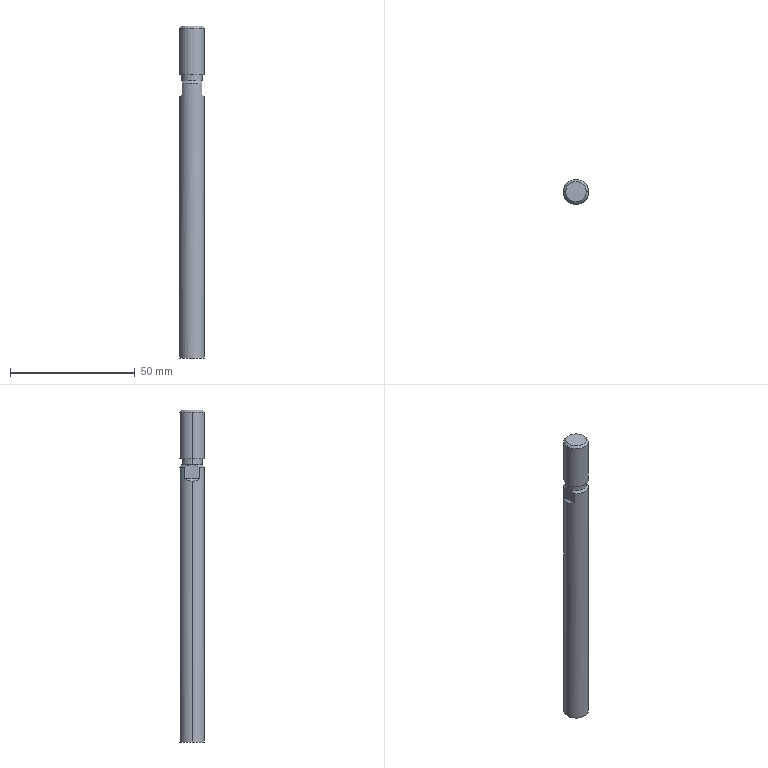Part | STEP file | rod_A_CDM2B25_100_C76_0_ | 1 solid | 19 faces | box 10 x 10 x 133 mm | volume 10311 mm3 | plane 9 | cylinder 6 | cone 4 | commonest cylinder face diameters 10 x4 8.16 x2
STEP:
#1=CARTESIAN_POINT('',(5.,0.,-101.));
#2=VERTEX_POINT('',#1);
#3=CARTESIAN_POINT('',(-5.,0.,-101.));
#4=VERTEX_POINT('',#3);
#5=CARTESIAN_POINT('',(0.,0.,-101.));
#6=DIRECTION('',(0.,0.,1.));
#7=DIRECTION('',(1.,0.,0.));
#8=AXIS2_PLACEMENT_3D('',#5,#6,#7);
#9=CIRCLE('',#8,5.);
#10=EDGE_CURVE('',#2,#4,#9,.T.);
#11=ORIENTED_EDGE('',*,*,#10,.T.);
#12=CARTESIAN_POINT('',(-5.,0.,3.5));
#13=VERTEX_POINT('',#12);
#14=CARTESIAN_POINT('',(-5.,0.,-101.));
#15=DIRECTION('',(0.,0.,1.));
#16=VECTOR('',#15,1000.);
#17=LINE('',#14,#16);
#18=EDGE_CURVE('',#4,#13,#17,.T.);
#19=ORIENTED_EDGE('',*,*,#18,.T.);
#20=CARTESIAN_POINT('',(-4.,3.,4.5));
#21=VERTEX_POINT('',#20);
#22=CARTESIAN_POINT('',(-5.,0.,3.5));
#23=CARTESIAN_POINT('',(-5.,1.091,3.5));
#24=CARTESIAN_POINT('',(-4.655,2.127,3.845));
#25=CARTESIAN_POINT('',(-4.,3.,4.5));
#26=(BOUNDED_CURVE()B_SPLINE_CURVE(3,(#22,#23,#24,#25),.UNSPECIFIED.,.F.,.T.)B_SPLINE_CURVE_WITH_KNOTS((4,4),(3.142,3.785),.UNSPECIFIED.)CURVE()GEOMETRIC_REPRESENTATION_ITEM()RATIONAL_B_SPLINE_CURVE((1.,0.9658,0.9658,1.))REPRESENTATION_ITEM(''));
#27=EDGE_CURVE('',#13,#21,#26,.T.);
#28=ORIENTED_EDGE('',*,*,#27,.T.);
#29=CARTESIAN_POINT('',(-4.,3.,9.08));
#30=VERTEX_POINT('',#29);
#31=CARTESIAN_POINT('',(-4.,3.,-101.));
#32=DIRECTION('',(0.,0.,1.));
#33=VECTOR('',#32,1000.);
#34=LINE('',#31,#33);
#35=EDGE_CURVE('',#21,#30,#34,.T.);
#36=ORIENTED_EDGE('',*,*,#35,.T.);
#37=CARTESIAN_POINT('',(4.,3.,9.08));
#38=VERTEX_POINT('',#37);
#39=CARTESIAN_POINT('',(0.,0.,9.08));
#40=DIRECTION('',(0.,0.,1.));
#41=DIRECTION('',(1.,0.,0.));
#42=AXIS2_PLACEMENT_3D('',#39,#40,#41);
#43=CIRCLE('',#42,5.);
#44=EDGE_CURVE('',#38,#30,#43,.T.);
#45=ORIENTED_EDGE('',*,*,#44,.F.);
#46=CARTESIAN_POINT('',(4.,3.,4.5));
#47=VERTEX_POINT('',#46);
#48=CARTESIAN_POINT('',(4.,3.,-101.));
#49=DIRECTION('',(0.,0.,-1.));
#50=VECTOR('',#49,1000.);
#51=LINE('',#48,#50);
#52=EDGE_CURVE('',#38,#47,#51,.T.);
#53=ORIENTED_EDGE('',*,*,#52,.T.);
#54=CARTESIAN_POINT('',(5.,0.,3.5));
#55=VERTEX_POINT('',#54);
#56=CARTESIAN_POINT('',(4.,3.,4.5));
#57=CARTESIAN_POINT('',(4.655,2.127,3.845));
#58=CARTESIAN_POINT('',(5.,1.091,3.5));
#59=CARTESIAN_POINT('',(5.,0.,3.5));
#60=(BOUNDED_CURVE()B_SPLINE_CURVE(3,(#56,#57,#58,#59),.UNSPECIFIED.,.F.,.T.)B_SPLINE_CURVE_WITH_KNOTS((4,4),(2.498,3.142),.UNSPECIFIED.)CURVE()GEOMETRIC_REPRESENTATION_ITEM()RATIONAL_B_SPLINE_CURVE((1.,0.9658,0.9658,1.))REPRESENTATION_ITEM(''));
#61=EDGE_CURVE('',#47,#55,#60,.T.);
#62=ORIENTED_EDGE('',*,*,#61,.T.);
#63=CARTESIAN_POINT('',(5.,0.,-101.));
#64=DIRECTION('',(0.,0.,1.));
#65=VECTOR('',#64,1000.);
#66=LINE('',#63,#65);
#67=EDGE_CURVE('',#2,#55,#66,.T.);
#68=ORIENTED_EDGE('',*,*,#67,.F.);
#69=EDGE_LOOP('',(#11,#19,#28,#36,#45,#53,#62,#68));
#70=FACE_OUTER_BOUND('',#69,.T.);
#71=CARTESIAN_POINT('',(0.,0.,-101.));
#72=DIRECTION('',(0.,0.,1.));
#73=DIRECTION('',(1.,0.,0.));
#74=AXIS2_PLACEMENT_3D('',#71,#72,#73);
#75=CYLINDRICAL_SURFACE('',#74,5.);
#76=ADVANCED_FACE('',(#70),#75,.T.);
#77=CARTESIAN_POINT('',(-4.,0.804,10.));
#78=VERTEX_POINT('',#77);
#79=CARTESIAN_POINT('',(-4.08,0.,10.));
#80=VERTEX_POINT('',#79);
#81=CARTESIAN_POINT('',(0.,0.,10.));
#82=DIRECTION('',(0.,0.,1.));
#83=DIRECTION('',(1.,0.,0.));
#84=AXIS2_PLACEMENT_3D('',#81,#82,#83);
#85=CIRCLE('',#84,4.08);
#86=EDGE_CURVE('',#78,#80,#85,.T.);
#87=ORIENTED_EDGE('',*,*,#86,.T.);
#88=CARTESIAN_POINT('',(-4.08,0.,12.5));
#89=VERTEX_POINT('',#88);
#90=CARTESIAN_POINT('',(-4.08,0.,-101.));
#91=DIRECTION('',(0.,0.,1.));
#92=VECTOR('',#91,1000.);
#93=LINE('',#90,#92);
#94=EDGE_CURVE('',#80,#89,#93,.T.);
#95=ORIENTED_EDGE('',*,*,#94,.T.);
#96=CARTESIAN_POINT('',(4.08,0.,12.5));
#97=VERTEX_POINT('',#96);
#98=CARTESIAN_POINT('',(0.,0.,12.5));
#99=DIRECTION('',(0.,0.,1.));
#100=DIRECTION('',(1.,0.,0.));
#101=AXIS2_PLACEMENT_3D('',#98,#99,#100);
#102=CIRCLE('',#101,4.08);
#103=EDGE_CURVE('',#97,#89,#102,.T.);
#104=ORIENTED_EDGE('',*,*,#103,.F.);
#105=CARTESIAN_POINT('',(4.08,0.,10.));
#106=VERTEX_POINT('',#105);
#107=CARTESIAN_POINT('',(4.08,0.,-101.));
#108=DIRECTION('',(0.,0.,1.));
#109=VECTOR('',#108,1000.);
#110=LINE('',#107,#109);
#111=EDGE_CURVE('',#106,#97,#110,.T.);
#112=ORIENTED_EDGE('',*,*,#111,.F.);
#113=CARTESIAN_POINT('',(4.,0.804,10.));
#114=VERTEX_POINT('',#113);
#115=CARTESIAN_POINT('',(0.,0.,10.));
#116=DIRECTION('',(0.,0.,1.));
#117=DIRECTION('',(1.,0.,0.));
#118=AXIS2_PLACEMENT_3D('',#115,#116,#117);
#119=CIRCLE('',#118,4.08);
#120=EDGE_CURVE('',#106,#114,#119,.T.);
#121=ORIENTED_EDGE('',*,*,#120,.T.);
#122=CARTESIAN_POINT('',(0.,0.,10.));
#123=DIRECTION('',(0.,0.,1.));
#124=DIRECTION('',(1.,0.,0.));
#125=AXIS2_PLACEMENT_3D('',#122,#123,#124);
#126=CIRCLE('',#125,4.08);
#127=EDGE_CURVE('',#114,#78,#126,.T.);
#128=ORIENTED_EDGE('',*,*,#127,.T.);
#129=EDGE_LOOP('',(#87,#95,#104,#112,#121,#128));
#130=FACE_OUTER_BOUND('',#129,.T.);
#131=CARTESIAN_POINT('',(0.,0.,-101.));
#132=DIRECTION('',(0.,0.,1.));
#133=DIRECTION('',(1.,0.,0.));
#134=AXIS2_PLACEMENT_3D('',#131,#132,#133);
#135=CYLINDRICAL_SURFACE('',#134,4.08);
#136=ADVANCED_FACE('',(#130),#135,.T.);
#137=CARTESIAN_POINT('',(5.,0.,12.5));
#138=VERTEX_POINT('',#137);
#139=CARTESIAN_POINT('',(-5.,0.,12.5));
#140=VERTEX_POINT('',#139);
#141=CARTESIAN_POINT('',(0.,0.,12.5));
#142=DIRECTION('',(0.,0.,1.));
#143=DIRECTION('',(1.,0.,0.));
#144=AXIS2_PLACEMENT_3D('',#141,#142,#143);
#145=CIRCLE('',#144,5.);
#146=EDGE_CURVE('',#138,#140,#145,.T.);
#147=ORIENTED_EDGE('',*,*,#146,.T.);
#148=CARTESIAN_POINT('',(-5.,0.,31.08));
#149=VERTEX_POINT('',#148);
#150=CARTESIAN_POINT('',(-5.,0.,-101.));
#151=DIRECTION('',(0.,0.,1.));
#152=VECTOR('',#151,1000.);
#153=LINE('',#150,#152);
#154=EDGE_CURVE('',#140,#149,#153,.T.);
#155=ORIENTED_EDGE('',*,*,#154,.T.);
#156=CARTESIAN_POINT('',(5.,0.,31.08));
#157=VERTEX_POINT('',#156);
#158=CARTESIAN_POINT('',(0.,0.,31.08));
#159=DIRECTION('',(0.,0.,1.));
#160=DIRECTION('',(1.,0.,0.));
#161=AXIS2_PLACEMENT_3D('',#158,#159,#160);
#162=CIRCLE('',#161,5.);
#163=EDGE_CURVE('',#157,#149,#162,.T.);
#164=ORIENTED_EDGE('',*,*,#163,.F.);
#165=CARTESIAN_POINT('',(5.,0.,-101.));
#166=DIRECTION('',(0.,0.,1.));
#167=VECTOR('',#166,1000.);
#168=LINE('',#165,#167);
#169=EDGE_CURVE('',#138,#157,#168,.T.);
#170=ORIENTED_EDGE('',*,*,#169,.F.);
#171=EDGE_LOOP('',(#147,#155,#164,#170));
#172=FACE_OUTER_BOUND('',#171,.T.);
#173=CARTESIAN_POINT('',(0.,0.,-101.));
#174=DIRECTION('',(0.,0.,1.));
#175=DIRECTION('',(1.,0.,0.));
#176=AXIS2_PLACEMENT_3D('',#173,#174,#175);
#177=CYLINDRICAL_SURFACE('',#176,5.);
#178=ADVANCED_FACE('',(#172),#177,.T.);
#179=CARTESIAN_POINT('',(4.08,0.,32.));
#180=VERTEX_POINT('',#179);
#181=CARTESIAN_POINT('',(-4.08,0.,32.));
#182=VERTEX_POINT('',#181);
#183=CARTESIAN_POINT('',(0.,0.,32.));
#184=DIRECTION('',(0.,0.,1.));
#185=DIRECTION('',(1.,0.,0.));
#186=AXIS2_PLACEMENT_3D('',#183,#184,#185);
#187=CIRCLE('',#186,4.08);
#188=EDGE_CURVE('',#180,#182,#187,.T.);
#189=ORIENTED_EDGE('',*,*,#188,.F.);
#190=CARTESIAN_POINT('',(5.,0.,31.08));
#191=DIRECTION('',(0.7071,0.,-0.7071));
#192=VECTOR('',#191,1000.);
#193=LINE('',#190,#192);
#194=EDGE_CURVE('',#180,#157,#193,.T.);
#195=ORIENTED_EDGE('',*,*,#194,.T.);
#196=ORIENTED_EDGE('',*,*,#163,.T.);
#197=CARTESIAN_POINT('',(-5.,0.,31.08));
#198=DIRECTION('',(-0.7071,0.,-0.7071));
#199=VECTOR('',#198,1000.);
#200=LINE('',#197,#199);
#201=EDGE_CURVE('',#182,#149,#200,.T.);
#202=ORIENTED_EDGE('',*,*,#201,.F.);
#203=EDGE_LOOP('',(#189,#195,#196,#202));
#204=FACE_OUTER_BOUND('',#203,.T.);
#205=CARTESIAN_POINT('',(0.,0.,31.08));
#206=DIRECTION('',(0.,0.,-1.));
#207=DIRECTION('',(-1.,0.,0.));
#208=AXIS2_PLACEMENT_3D('',#205,#206,#207);
#209=CONICAL_SURFACE('',#208,5.,0.7854);
#210=ADVANCED_FACE('',(#204),#209,.T.);
#211=ORIENTED_EDGE('',*,*,#44,.T.);
#212=CARTESIAN_POINT('',(-4.,3.,9.08));
#213=CARTESIAN_POINT('',(-4.,2.657,9.286));
#214=CARTESIAN_POINT('',(-4.,2.306,9.474));
#215=CARTESIAN_POINT('',(-4.,1.576,9.793));
#216=CARTESIAN_POINT('',(-4.,1.193,9.923));
#217=CARTESIAN_POINT('',(-4.,0.804,10.));
#218=B_SPLINE_CURVE_WITH_KNOTS('',3,(#212,#213,#214,#215,#216,#217),.UNSPECIFIED.,.F.,.F.,(4,2,4),(0.00946,0.01066,0.01185),.UNSPECIFIED.);
#219=EDGE_CURVE('',#30,#78,#218,.T.);
#220=ORIENTED_EDGE('',*,*,#219,.T.);
#221=ORIENTED_EDGE('',*,*,#127,.F.);
#222=CARTESIAN_POINT('',(4.,0.804,10.));
#223=CARTESIAN_POINT('',(4.,1.195,9.923));
#224=CARTESIAN_POINT('',(4.,1.58,9.792));
#225=CARTESIAN_POINT('',(4.,2.311,9.472));
#226=CARTESIAN_POINT('',(4.,2.66,9.284));
#227=CARTESIAN_POINT('',(4.,3.,9.08));
#228=B_SPLINE_CURVE_WITH_KNOTS('',3,(#222,#223,#224,#225,#226,#227),.UNSPECIFIED.,.F.,.F.,(4,2,4),(0.01347,0.01467,0.01588),.UNSPECIFIED.);
#229=EDGE_CURVE('',#114,#38,#228,.T.);
#230=ORIENTED_EDGE('',*,*,#229,.T.);
#231=EDGE_LOOP('',(#211,#220,#221,#230));
#232=FACE_OUTER_BOUND('',#231,.T.);
#233=CARTESIAN_POINT('',(0.,0.,9.08));
#234=DIRECTION('',(0.,0.,-1.));
#235=DIRECTION('',(-1.,0.,0.));
#236=AXIS2_PLACEMENT_3D('',#233,#234,#235);
#237=CONICAL_SURFACE('',#236,5.,0.7854);
#238=ADVANCED_FACE('',(#232),#237,.T.);
#239=CARTESIAN_POINT('',(0.,0.,32.));
#240=DIRECTION('',(0.,0.,1.));
#241=DIRECTION('',(1.,0.,0.));
#242=AXIS2_PLACEMENT_3D('',#239,#240,#241);
#243=CIRCLE('',#242,4.08);
#244=EDGE_CURVE('',#182,#180,#243,.T.);
#245=ORIENTED_EDGE('',*,*,#244,.T.);
#246=ORIENTED_EDGE('',*,*,#188,.T.);
#247=EDGE_LOOP('',(#245,#246));
#248=FACE_OUTER_BOUND('',#247,.T.);
#249=CARTESIAN_POINT('',(0.,0.,32.));
#250=DIRECTION('',(0.,0.,-1.));
#251=DIRECTION('',(-1.,0.,0.));
#252=AXIS2_PLACEMENT_3D('',#249,#250,#251);
#253=PLANE('',#252);
#254=ADVANCED_FACE('',(#248),#253,.F.);
#255=ORIENTED_EDGE('',*,*,#194,.F.);
#256=ORIENTED_EDGE('',*,*,#244,.F.);
#257=ORIENTED_EDGE('',*,*,#201,.T.);
#258=CARTESIAN_POINT('',(0.,0.,31.08));
#259=DIRECTION('',(0.,0.,1.));
#260=DIRECTION('',(1.,0.,0.));
#261=AXIS2_PLACEMENT_3D('',#258,#259,#260);
#262=CIRCLE('',#261,5.);
#263=EDGE_CURVE('',#149,#157,#262,.T.);
#264=ORIENTED_EDGE('',*,*,#263,.T.);
#265=EDGE_LOOP('',(#255,#256,#257,#264));
#266=FACE_OUTER_BOUND('',#265,.T.);
#267=CARTESIAN_POINT('',(0.,0.,31.08));
#268=DIRECTION('',(0.,0.,-1.));
#269=DIRECTION('',(-1.,0.,0.));
#270=AXIS2_PLACEMENT_3D('',#267,#268,#269);
#271=CONICAL_SURFACE('',#270,5.,0.7854);
#272=ADVANCED_FACE('',(#266),#271,.T.);
#273=ORIENTED_EDGE('',*,*,#154,.F.);
#274=CARTESIAN_POINT('',(0.,0.,12.5));
#275=DIRECTION('',(0.,0.,1.));
#276=DIRECTION('',(1.,0.,0.));
#277=AXIS2_PLACEMENT_3D('',#274,#275,#276);
#278=CIRCLE('',#277,5.);
#279=EDGE_CURVE('',#140,#138,#278,.T.);
#280=ORIENTED_EDGE('',*,*,#279,.T.);
#281=ORIENTED_EDGE('',*,*,#169,.T.);
#282=ORIENTED_EDGE('',*,*,#263,.F.);
#283=EDGE_LOOP('',(#273,#280,#281,#282));
#284=FACE_OUTER_BOUND('',#283,.T.);
#285=CARTESIAN_POINT('',(0.,0.,-101.));
#286=DIRECTION('',(0.,0.,1.));
#287=DIRECTION('',(1.,0.,0.));
#288=AXIS2_PLACEMENT_3D('',#285,#286,#287);
#289=CYLINDRICAL_SURFACE('',#288,5.);
#290=ADVANCED_FACE('',(#284),#289,.T.);
#291=ORIENTED_EDGE('',*,*,#146,.F.);
#292=ORIENTED_EDGE('',*,*,#279,.F.);
#293=EDGE_LOOP('',(#291,#292));
#294=FACE_OUTER_BOUND('',#293,.T.);
#295=ORIENTED_EDGE('',*,*,#103,.T.);
#296=CARTESIAN_POINT('',(0.,0.,12.5));
#297=DIRECTION('',(0.,0.,1.));
#298=DIRECTION('',(1.,0.,0.));
#299=AXIS2_PLACEMENT_3D('',#296,#297,#298);
#300=CIRCLE('',#299,4.08);
#301=EDGE_CURVE('',#89,#97,#300,.T.);
#302=ORIENTED_EDGE('',*,*,#301,.T.);
#303=EDGE_LOOP('',(#295,#302));
#304=FACE_BOUND('',#303,.T.);
#305=CARTESIAN_POINT('',(0.,5.,12.5));
#306=DIRECTION('',(0.,0.,1.));
#307=DIRECTION('',(1.,0.,0.));
#308=AXIS2_PLACEMENT_3D('',#305,#306,#307);
#309=PLANE('',#308);
#310=ADVANCED_FACE('',(#294,#304),#309,.F.);
#311=ORIENTED_EDGE('',*,*,#94,.F.);
#312=CARTESIAN_POINT('',(-4.,-0.804,10.));
#313=VERTEX_POINT('',#312);
#314=CARTESIAN_POINT('',(0.,0.,10.));
#315=DIRECTION('',(0.,0.,1.));
#316=DIRECTION('',(1.,0.,0.));
#317=AXIS2_PLACEMENT_3D('',#314,#315,#316);
#318=CIRCLE('',#317,4.08);
#319=EDGE_CURVE('',#80,#313,#318,.T.);
#320=ORIENTED_EDGE('',*,*,#319,.T.);
#321=CARTESIAN_POINT('',(4.,-0.804,10.));
#322=VERTEX_POINT('',#321);
#323=CARTESIAN_POINT('',(0.,0.,10.));
#324=DIRECTION('',(0.,0.,1.));
#325=DIRECTION('',(1.,0.,0.));
#326=AXIS2_PLACEMENT_3D('',#323,#324,#325);
#327=CIRCLE('',#326,4.08);
#328=EDGE_CURVE('',#313,#322,#327,.T.);
#329=ORIENTED_EDGE('',*,*,#328,.T.);
#330=CARTESIAN_POINT('',(0.,0.,10.));
#331=DIRECTION('',(0.,0.,1.));
#332=DIRECTION('',(1.,0.,0.));
#333=AXIS2_PLACEMENT_3D('',#330,#331,#332);
#334=CIRCLE('',#333,4.08);
#335=EDGE_CURVE('',#322,#106,#334,.T.);
#336=ORIENTED_EDGE('',*,*,#335,.T.);
#337=ORIENTED_EDGE('',*,*,#111,.T.);
#338=ORIENTED_EDGE('',*,*,#301,.F.);
#339=EDGE_LOOP('',(#311,#320,#329,#336,#337,#338));
#340=FACE_OUTER_BOUND('',#339,.T.);
#341=CARTESIAN_POINT('',(0.,0.,-101.));
#342=DIRECTION('',(0.,0.,1.));
#343=DIRECTION('',(1.,0.,0.));
#344=AXIS2_PLACEMENT_3D('',#341,#342,#343);
#345=CYLINDRICAL_SURFACE('',#344,4.08);
#346=ADVANCED_FACE('',(#340),#345,.T.);
#347=ORIENTED_EDGE('',*,*,#328,.F.);
#348=CARTESIAN_POINT('',(-4.,-3.,9.08));
#349=VERTEX_POINT('',#348);
#350=CARTESIAN_POINT('',(-4.,-0.804,10.));
#351=CARTESIAN_POINT('',(-4.,-1.195,9.923));
#352=CARTESIAN_POINT('',(-4.,-1.58,9.792));
#353=CARTESIAN_POINT('',(-4.,-2.311,9.472));
#354=CARTESIAN_POINT('',(-4.,-2.66,9.284));
#355=CARTESIAN_POINT('',(-4.,-3.,9.08));
#356=B_SPLINE_CURVE_WITH_KNOTS('',3,(#350,#351,#352,#353,#354,#355),.UNSPECIFIED.,.F.,.F.,(4,2,4),(0.01347,0.01467,0.01588),.UNSPECIFIED.);
#357=EDGE_CURVE('',#313,#349,#356,.T.);
#358=ORIENTED_EDGE('',*,*,#357,.T.);
#359=CARTESIAN_POINT('',(4.,-3.,9.08));
#360=VERTEX_POINT('',#359);
#361=CARTESIAN_POINT('',(0.,0.,9.08));
#362=DIRECTION('',(0.,0.,1.));
#363=DIRECTION('',(1.,0.,0.));
#364=AXIS2_PLACEMENT_3D('',#361,#362,#363);
#365=CIRCLE('',#364,5.);
#366=EDGE_CURVE('',#349,#360,#365,.T.);
#367=ORIENTED_EDGE('',*,*,#366,.T.);
#368=CARTESIAN_POINT('',(4.,-3.,9.08));
#369=CARTESIAN_POINT('',(4.,-2.657,9.286));
#370=CARTESIAN_POINT('',(4.,-2.306,9.474));
#371=CARTESIAN_POINT('',(4.,-1.576,9.793));
#372=CARTESIAN_POINT('',(4.,-1.193,9.923));
#373=CARTESIAN_POINT('',(4.,-0.804,10.));
#374=B_SPLINE_CURVE_WITH_KNOTS('',3,(#368,#369,#370,#371,#372,#373),.UNSPECIFIED.,.F.,.F.,(4,2,4),(0.00946,0.01066,0.01185),.UNSPECIFIED.);
#375=EDGE_CURVE('',#360,#322,#374,.T.);
#376=ORIENTED_EDGE('',*,*,#375,.T.);
#377=EDGE_LOOP('',(#347,#358,#367,#376));
#378=FACE_OUTER_BOUND('',#377,.T.);
#379=CARTESIAN_POINT('',(0.,0.,9.08));
#380=DIRECTION('',(0.,0.,-1.));
#381=DIRECTION('',(-1.,0.,0.));
#382=AXIS2_PLACEMENT_3D('',#379,#380,#381);
#383=CONICAL_SURFACE('',#382,5.,0.7854);
#384=ADVANCED_FACE('',(#378),#383,.T.);
#385=ORIENTED_EDGE('',*,*,#18,.F.);
#386=CARTESIAN_POINT('',(0.,0.,-101.));
#387=DIRECTION('',(0.,0.,1.));
#388=DIRECTION('',(1.,0.,0.));
#389=AXIS2_PLACEMENT_3D('',#386,#387,#388);
#390=CIRCLE('',#389,5.);
#391=EDGE_CURVE('',#4,#2,#390,.T.);
#392=ORIENTED_EDGE('',*,*,#391,.T.);
#393=ORIENTED_EDGE('',*,*,#67,.T.);
#394=CARTESIAN_POINT('',(4.,-3.,4.5));
#395=VERTEX_POINT('',#394);
#396=CARTESIAN_POINT('',(5.,0.,3.5));
#397=CARTESIAN_POINT('',(5.,-1.091,3.5));
#398=CARTESIAN_POINT('',(4.655,-2.127,3.845));
#399=CARTESIAN_POINT('',(4.,-3.,4.5));
#400=(BOUNDED_CURVE()B_SPLINE_CURVE(3,(#396,#397,#398,#399),.UNSPECIFIED.,.F.,.F.)B_SPLINE_CURVE_WITH_KNOTS((4,4),(3.142,3.785),.UNSPECIFIED.)CURVE()GEOMETRIC_REPRESENTATION_ITEM()RATIONAL_B_SPLINE_CURVE((1.,0.9658,0.9658,1.))REPRESENTATION_ITEM(''));
#401=EDGE_CURVE('',#55,#395,#400,.T.);
#402=ORIENTED_EDGE('',*,*,#401,.T.);
#403=CARTESIAN_POINT('',(4.,-3.,-101.));
#404=DIRECTION('',(0.,0.,1.));
#405=VECTOR('',#404,1000.);
#406=LINE('',#403,#405);
#407=EDGE_CURVE('',#395,#360,#406,.T.);
#408=ORIENTED_EDGE('',*,*,#407,.T.);
#409=ORIENTED_EDGE('',*,*,#366,.F.);
#410=CARTESIAN_POINT('',(-4.,-3.,4.5));
#411=VERTEX_POINT('',#410);
#412=CARTESIAN_POINT('',(-4.,-3.,-101.));
#413=DIRECTION('',(0.,0.,-1.));
#414=VECTOR('',#413,1000.);
#415=LINE('',#412,#414);
#416=EDGE_CURVE('',#349,#411,#415,.T.);
#417=ORIENTED_EDGE('',*,*,#416,.T.);
#418=CARTESIAN_POINT('',(-4.,-3.,4.5));
#419=CARTESIAN_POINT('',(-4.655,-2.127,3.845));
#420=CARTESIAN_POINT('',(-5.,-1.091,3.5));
#421=CARTESIAN_POINT('',(-5.,0.,3.5));
#422=(BOUNDED_CURVE()B_SPLINE_CURVE(3,(#418,#419,#420,#421),.UNSPECIFIED.,.F.,.F.)B_SPLINE_CURVE_WITH_KNOTS((4,4),(2.498,3.142),.UNSPECIFIED.)CURVE()GEOMETRIC_REPRESENTATION_ITEM()RATIONAL_B_SPLINE_CURVE((1.,0.9658,0.9658,1.))REPRESENTATION_ITEM(''));
#423=EDGE_CURVE('',#411,#13,#422,.T.);
#424=ORIENTED_EDGE('',*,*,#423,.T.);
#425=EDGE_LOOP('',(#385,#392,#393,#402,#408,#409,#417,#424));
#426=FACE_OUTER_BOUND('',#425,.T.);
#427=CARTESIAN_POINT('',(0.,0.,-101.));
#428=DIRECTION('',(0.,0.,1.));
#429=DIRECTION('',(1.,0.,0.));
#430=AXIS2_PLACEMENT_3D('',#427,#428,#429);
#431=CYLINDRICAL_SURFACE('',#430,5.);
#432=ADVANCED_FACE('',(#426),#431,.T.);
#433=ORIENTED_EDGE('',*,*,#10,.F.);
#434=ORIENTED_EDGE('',*,*,#391,.F.);
#435=EDGE_LOOP('',(#433,#434));
#436=FACE_OUTER_BOUND('',#435,.T.);
#437=CARTESIAN_POINT('',(0.,5.,-101.));
#438=DIRECTION('',(0.,0.,1.));
#439=DIRECTION('',(1.,0.,0.));
#440=AXIS2_PLACEMENT_3D('',#437,#438,#439);
#441=PLANE('',#440);
#442=ADVANCED_FACE('',(#436),#441,.F.);
#443=CARTESIAN_POINT('',(4.,-10.,10.));
#444=DIRECTION('',(0.,1.,0.));
#445=VECTOR('',#444,1000.);
#446=LINE('',#443,#445);
#447=EDGE_CURVE('',#322,#114,#446,.T.);
#448=ORIENTED_EDGE('',*,*,#447,.T.);
#449=ORIENTED_EDGE('',*,*,#120,.F.);
#450=ORIENTED_EDGE('',*,*,#335,.F.);
#451=EDGE_LOOP('',(#448,#449,#450));
#452=FACE_OUTER_BOUND('',#451,.T.);
#453=CARTESIAN_POINT('',(4.,-10.,10.));
#454=DIRECTION('',(0.,0.,1.));
#455=DIRECTION('',(1.,0.,0.));
#456=AXIS2_PLACEMENT_3D('',#453,#454,#455);
#457=PLANE('',#456);
#458=ADVANCED_FACE('',(#452),#457,.F.);
#459=ORIENTED_EDGE('',*,*,#407,.F.);
#460=CARTESIAN_POINT('',(4.,-10.,4.5));
#461=DIRECTION('',(0.,1.,0.));
#462=VECTOR('',#461,1000.);
#463=LINE('',#460,#462);
#464=EDGE_CURVE('',#395,#47,#463,.T.);
#465=ORIENTED_EDGE('',*,*,#464,.T.);
#466=ORIENTED_EDGE('',*,*,#52,.F.);
#467=ORIENTED_EDGE('',*,*,#229,.F.);
#468=ORIENTED_EDGE('',*,*,#447,.F.);
#469=ORIENTED_EDGE('',*,*,#375,.F.);
#470=EDGE_LOOP('',(#459,#465,#466,#467,#468,#469));
#471=FACE_OUTER_BOUND('',#470,.T.);
#472=CARTESIAN_POINT('',(4.,-10.,4.5));
#473=DIRECTION('',(-1.,0.,0.));
#474=DIRECTION('',(0.,0.,1.));
#475=AXIS2_PLACEMENT_3D('',#472,#473,#474);
#476=PLANE('',#475);
#477=ADVANCED_FACE('',(#471),#476,.F.);
#478=ORIENTED_EDGE('',*,*,#464,.F.);
#479=ORIENTED_EDGE('',*,*,#401,.F.);
#480=ORIENTED_EDGE('',*,*,#61,.F.);
#481=EDGE_LOOP('',(#478,#479,#480));
#482=FACE_OUTER_BOUND('',#481,.T.);
#483=CARTESIAN_POINT('',(5.,-10.,3.5));
#484=DIRECTION('',(-0.7071,0.,-0.7071));
#485=DIRECTION('',(-0.7071,0.,0.7071));
#486=AXIS2_PLACEMENT_3D('',#483,#484,#485);
#487=PLANE('',#486);
#488=ADVANCED_FACE('',(#482),#487,.F.);
#489=CARTESIAN_POINT('',(-4.,-10.,10.));
#490=DIRECTION('',(0.,1.,0.));
#491=VECTOR('',#490,1000.);
#492=LINE('',#489,#491);
#493=EDGE_CURVE('',#313,#78,#492,.T.);
#494=ORIENTED_EDGE('',*,*,#493,.F.);
#495=ORIENTED_EDGE('',*,*,#319,.F.);
#496=ORIENTED_EDGE('',*,*,#86,.F.);
#497=EDGE_LOOP('',(#494,#495,#496));
#498=FACE_OUTER_BOUND('',#497,.T.);
#499=CARTESIAN_POINT('',(-7.,-10.,10.));
#500=DIRECTION('',(0.,0.,1.));
#501=DIRECTION('',(1.,0.,0.));
#502=AXIS2_PLACEMENT_3D('',#499,#500,#501);
#503=PLANE('',#502);
#504=ADVANCED_FACE('',(#498),#503,.F.);
#505=CARTESIAN_POINT('',(-4.,-10.,4.5));
#506=DIRECTION('',(0.,1.,0.));
#507=VECTOR('',#506,1000.);
#508=LINE('',#505,#507);
#509=EDGE_CURVE('',#411,#21,#508,.T.);
#510=ORIENTED_EDGE('',*,*,#509,.T.);
#511=ORIENTED_EDGE('',*,*,#27,.F.);
#512=ORIENTED_EDGE('',*,*,#423,.F.);
#513=EDGE_LOOP('',(#510,#511,#512));
#514=FACE_OUTER_BOUND('',#513,.T.);
#515=CARTESIAN_POINT('',(-4.,-10.,4.5));
#516=DIRECTION('',(0.7071,0.,-0.7071));
#517=DIRECTION('',(-0.7071,0.,-0.7071));
#518=AXIS2_PLACEMENT_3D('',#515,#516,#517);
#519=PLANE('',#518);
#520=ADVANCED_FACE('',(#514),#519,.F.);
#521=ORIENTED_EDGE('',*,*,#35,.F.);
#522=ORIENTED_EDGE('',*,*,#509,.F.);
#523=ORIENTED_EDGE('',*,*,#416,.F.);
#524=ORIENTED_EDGE('',*,*,#357,.F.);
#525=ORIENTED_EDGE('',*,*,#493,.T.);
#526=ORIENTED_EDGE('',*,*,#219,.F.);
#527=EDGE_LOOP('',(#521,#522,#523,#524,#525,#526));
#528=FACE_OUTER_BOUND('',#527,.T.);
#529=CARTESIAN_POINT('',(-4.,-10.,10.));
#530=DIRECTION('',(1.,0.,0.));
#531=DIRECTION('',(0.,0.,-1.));
#532=AXIS2_PLACEMENT_3D('',#529,#530,#531);
#533=PLANE('',#532);
#534=ADVANCED_FACE('',(#528),#533,.F.);
#535=CLOSED_SHELL('',(#76,#136,#178,#210,#238,#254,#272,#290,#310,#346,#384,#432,#442,#458,#477,#488,#504,#520,#534));
#536=MANIFOLD_SOLID_BREP('',#535);
#537=CARTESIAN_POINT('',(0.,0.,0.));
#538=DIRECTION('',(0.,0.,1.));
#539=DIRECTION('',(1.,0.,0.));
#540=AXIS2_PLACEMENT_3D('',#537,#538,#539);
#541=(LENGTH_UNIT()NAMED_UNIT(*)SI_UNIT(.MILLI.,.METRE.));
#542=UNCERTAINTY_MEASURE_WITH_UNIT(LENGTH_MEASURE(0.00001),#541,'','');
#543=(NAMED_UNIT(*)PLANE_ANGLE_UNIT()SI_UNIT($,.RADIAN.));
#544=(NAMED_UNIT(*)SI_UNIT($,.STERADIAN.)SOLID_ANGLE_UNIT());
#545=(GEOMETRIC_REPRESENTATION_CONTEXT(3)GLOBAL_UNCERTAINTY_ASSIGNED_CONTEXT((#542))GLOBAL_UNIT_ASSIGNED_CONTEXT((#541,#543,#544))REPRESENTATION_CONTEXT('',''));
#546=ADVANCED_BREP_SHAPE_REPRESENTATION('',(#536,#540),#545);